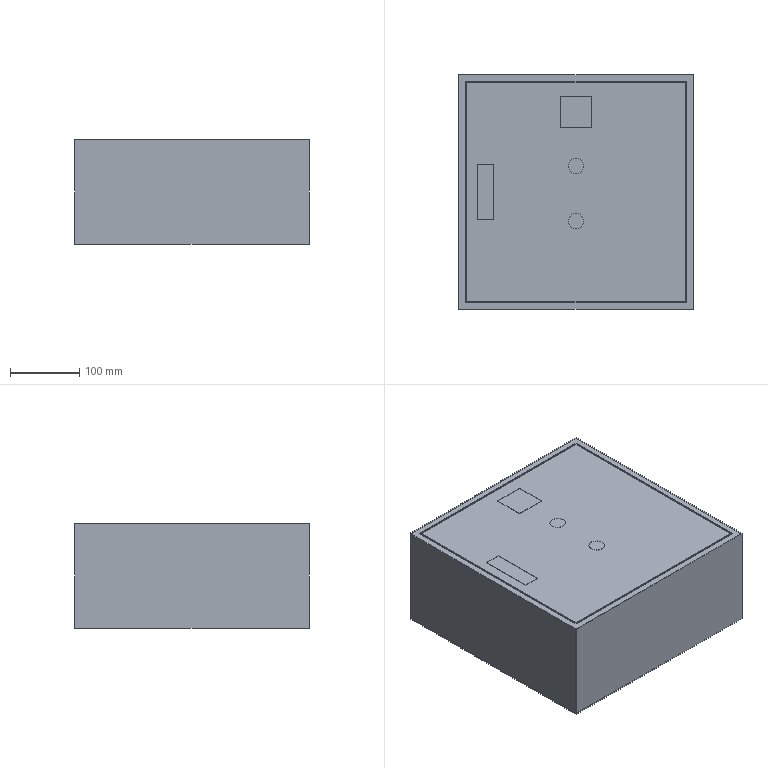Part | SolidWorks | features ICE 2, Extrusion 1, Shell 1 | 1 solid | 38 faces | box 340 x 340 x 151 mm | volume 586961 mm3 | plane 34 | cylinder 4 | commonest cylinder face diameters 22.5 x4
STEP:
#1=CARTESIAN_POINT('',(158.75,127.5,150.5));
#2=VERTEX_POINT('',#1);
#3=CARTESIAN_POINT('',(181.25,127.5,150.5));
#4=VERTEX_POINT('',#3);
#5=CARTESIAN_POINT('',(170.,127.5,150.5));
#6=DIRECTION('',(0.,0.,1.));
#7=DIRECTION('',(1.,0.,0.));
#8=AXIS2_PLACEMENT_3D('',#5,#6,#7);
#9=CIRCLE('',#8,11.25);
#10=EDGE_CURVE('',#2,#4,#9,.T.);
#11=ORIENTED_EDGE('',*,*,#10,.F.);
#12=CARTESIAN_POINT('',(158.75,127.5,151.));
#13=VERTEX_POINT('',#12);
#14=CARTESIAN_POINT('',(158.75,127.5,150.5));
#15=DIRECTION('',(0.,0.,1.));
#16=VECTOR('',#15,1000.);
#17=LINE('',#14,#16);
#18=EDGE_CURVE('',#2,#13,#17,.T.);
#19=ORIENTED_EDGE('',*,*,#18,.T.);
#20=CARTESIAN_POINT('',(181.25,127.5,151.));
#21=VERTEX_POINT('',#20);
#22=CARTESIAN_POINT('',(170.,127.5,151.));
#23=DIRECTION('',(0.,0.,1.));
#24=DIRECTION('',(1.,0.,0.));
#25=AXIS2_PLACEMENT_3D('',#22,#23,#24);
#26=CIRCLE('',#25,11.25);
#27=EDGE_CURVE('',#13,#21,#26,.T.);
#28=ORIENTED_EDGE('',*,*,#27,.T.);
#29=CARTESIAN_POINT('',(181.25,127.5,150.5));
#30=DIRECTION('',(0.,0.,1.));
#31=VECTOR('',#30,1000.);
#32=LINE('',#29,#31);
#33=EDGE_CURVE('',#4,#21,#32,.T.);
#34=ORIENTED_EDGE('',*,*,#33,.F.);
#35=EDGE_LOOP('',(#11,#19,#28,#34));
#36=FACE_OUTER_BOUND('',#35,.T.);
#37=CARTESIAN_POINT('',(170.,127.5,150.5));
#38=DIRECTION('',(0.,0.,1.));
#39=DIRECTION('',(1.,0.,0.));
#40=AXIS2_PLACEMENT_3D('',#37,#38,#39);
#41=CYLINDRICAL_SURFACE('',#40,11.25);
#42=ADVANCED_FACE('',(#36),#41,.F.);
#43=CARTESIAN_POINT('',(158.75,207.5,150.5));
#44=VERTEX_POINT('',#43);
#45=CARTESIAN_POINT('',(181.25,207.5,150.5));
#46=VERTEX_POINT('',#45);
#47=CARTESIAN_POINT('',(170.,207.5,150.5));
#48=DIRECTION('',(0.,0.,1.));
#49=DIRECTION('',(1.,0.,0.));
#50=AXIS2_PLACEMENT_3D('',#47,#48,#49);
#51=CIRCLE('',#50,11.25);
#52=EDGE_CURVE('',#44,#46,#51,.T.);
#53=ORIENTED_EDGE('',*,*,#52,.F.);
#54=CARTESIAN_POINT('',(158.75,207.5,151.));
#55=VERTEX_POINT('',#54);
#56=CARTESIAN_POINT('',(158.75,207.5,150.5));
#57=DIRECTION('',(0.,0.,1.));
#58=VECTOR('',#57,1000.);
#59=LINE('',#56,#58);
#60=EDGE_CURVE('',#44,#55,#59,.T.);
#61=ORIENTED_EDGE('',*,*,#60,.T.);
#62=CARTESIAN_POINT('',(181.25,207.5,151.));
#63=VERTEX_POINT('',#62);
#64=CARTESIAN_POINT('',(170.,207.5,151.));
#65=DIRECTION('',(0.,0.,1.));
#66=DIRECTION('',(1.,0.,0.));
#67=AXIS2_PLACEMENT_3D('',#64,#65,#66);
#68=CIRCLE('',#67,11.25);
#69=EDGE_CURVE('',#55,#63,#68,.T.);
#70=ORIENTED_EDGE('',*,*,#69,.T.);
#71=CARTESIAN_POINT('',(181.25,207.5,150.5));
#72=DIRECTION('',(0.,0.,1.));
#73=VECTOR('',#72,1000.);
#74=LINE('',#71,#73);
#75=EDGE_CURVE('',#46,#63,#74,.T.);
#76=ORIENTED_EDGE('',*,*,#75,.F.);
#77=EDGE_LOOP('',(#53,#61,#70,#76));
#78=FACE_OUTER_BOUND('',#77,.T.);
#79=CARTESIAN_POINT('',(170.,207.5,150.5));
#80=DIRECTION('',(0.,0.,1.));
#81=DIRECTION('',(1.,0.,0.));
#82=AXIS2_PLACEMENT_3D('',#79,#80,#81);
#83=CYLINDRICAL_SURFACE('',#82,11.25);
#84=ADVANCED_FACE('',(#78),#83,.F.);
#85=CARTESIAN_POINT('',(0.,340.,0.));
#86=VERTEX_POINT('',#85);
#87=CARTESIAN_POINT('',(0.,0.,0.));
#88=VERTEX_POINT('',#87);
#89=CARTESIAN_POINT('',(0.,0.,0.));
#90=DIRECTION('',(0.,-1.,0.));
#91=VECTOR('',#90,1000.);
#92=LINE('',#89,#91);
#93=EDGE_CURVE('',#86,#88,#92,.T.);
#94=ORIENTED_EDGE('',*,*,#93,.T.);
#95=CARTESIAN_POINT('',(0.,0.,151.));
#96=VERTEX_POINT('',#95);
#97=CARTESIAN_POINT('',(0.,0.,150.));
#98=DIRECTION('',(0.,0.,-1.));
#99=VECTOR('',#98,1000.);
#100=LINE('',#97,#99);
#101=EDGE_CURVE('',#96,#88,#100,.T.);
#102=ORIENTED_EDGE('',*,*,#101,.F.);
#103=CARTESIAN_POINT('',(0.,340.,151.));
#104=VERTEX_POINT('',#103);
#105=CARTESIAN_POINT('',(0.,340.,151.));
#106=DIRECTION('',(0.,-1.,0.));
#107=VECTOR('',#106,1000.);
#108=LINE('',#105,#107);
#109=EDGE_CURVE('',#104,#96,#108,.T.);
#110=ORIENTED_EDGE('',*,*,#109,.F.);
#111=CARTESIAN_POINT('',(0.,340.,150.));
#112=DIRECTION('',(0.,0.,-1.));
#113=VECTOR('',#112,1000.);
#114=LINE('',#111,#113);
#115=EDGE_CURVE('',#104,#86,#114,.T.);
#116=ORIENTED_EDGE('',*,*,#115,.T.);
#117=EDGE_LOOP('',(#94,#102,#110,#116));
#118=FACE_OUTER_BOUND('',#117,.T.);
#119=CARTESIAN_POINT('',(0.,0.,150.));
#120=DIRECTION('',(1.,0.,0.));
#121=DIRECTION('',(0.,0.,-1.));
#122=AXIS2_PLACEMENT_3D('',#119,#120,#121);
#123=PLANE('',#122);
#124=ADVANCED_FACE('',(#118),#123,.F.);
#125=CARTESIAN_POINT('',(340.,0.,0.));
#126=VERTEX_POINT('',#125);
#127=CARTESIAN_POINT('',(0.,0.,0.));
#128=DIRECTION('',(1.,0.,0.));
#129=VECTOR('',#128,1000.);
#130=LINE('',#127,#129);
#131=EDGE_CURVE('',#88,#126,#130,.T.);
#132=ORIENTED_EDGE('',*,*,#131,.T.);
#133=CARTESIAN_POINT('',(340.,0.,151.));
#134=VERTEX_POINT('',#133);
#135=CARTESIAN_POINT('',(340.,0.,150.));
#136=DIRECTION('',(0.,0.,-1.));
#137=VECTOR('',#136,1000.);
#138=LINE('',#135,#137);
#139=EDGE_CURVE('',#134,#126,#138,.T.);
#140=ORIENTED_EDGE('',*,*,#139,.F.);
#141=CARTESIAN_POINT('',(0.,0.,151.));
#142=DIRECTION('',(1.,0.,0.));
#143=VECTOR('',#142,1000.);
#144=LINE('',#141,#143);
#145=EDGE_CURVE('',#96,#134,#144,.T.);
#146=ORIENTED_EDGE('',*,*,#145,.F.);
#147=ORIENTED_EDGE('',*,*,#101,.T.);
#148=EDGE_LOOP('',(#132,#140,#146,#147));
#149=FACE_OUTER_BOUND('',#148,.T.);
#150=CARTESIAN_POINT('',(0.,0.,150.));
#151=DIRECTION('',(0.,1.,0.));
#152=DIRECTION('',(0.,0.,1.));
#153=AXIS2_PLACEMENT_3D('',#150,#151,#152);
#154=PLANE('',#153);
#155=ADVANCED_FACE('',(#149),#154,.F.);
#156=CARTESIAN_POINT('',(340.,340.,0.));
#157=VERTEX_POINT('',#156);
#158=CARTESIAN_POINT('',(340.,0.,0.));
#159=DIRECTION('',(0.,1.,0.));
#160=VECTOR('',#159,1000.);
#161=LINE('',#158,#160);
#162=EDGE_CURVE('',#126,#157,#161,.T.);
#163=ORIENTED_EDGE('',*,*,#162,.T.);
#164=CARTESIAN_POINT('',(340.,340.,151.));
#165=VERTEX_POINT('',#164);
#166=CARTESIAN_POINT('',(340.,340.,150.));
#167=DIRECTION('',(0.,0.,-1.));
#168=VECTOR('',#167,1000.);
#169=LINE('',#166,#168);
#170=EDGE_CURVE('',#165,#157,#169,.T.);
#171=ORIENTED_EDGE('',*,*,#170,.F.);
#172=CARTESIAN_POINT('',(340.,0.,151.));
#173=DIRECTION('',(0.,1.,0.));
#174=VECTOR('',#173,1000.);
#175=LINE('',#172,#174);
#176=EDGE_CURVE('',#134,#165,#175,.T.);
#177=ORIENTED_EDGE('',*,*,#176,.F.);
#178=ORIENTED_EDGE('',*,*,#139,.T.);
#179=EDGE_LOOP('',(#163,#171,#177,#178));
#180=FACE_OUTER_BOUND('',#179,.T.);
#181=CARTESIAN_POINT('',(340.,0.,150.));
#182=DIRECTION('',(-1.,0.,0.));
#183=DIRECTION('',(0.,0.,1.));
#184=AXIS2_PLACEMENT_3D('',#181,#182,#183);
#185=PLANE('',#184);
#186=ADVANCED_FACE('',(#180),#185,.F.);
#187=CARTESIAN_POINT('',(0.,340.,0.));
#188=DIRECTION('',(-1.,0.,0.));
#189=VECTOR('',#188,1000.);
#190=LINE('',#187,#189);
#191=EDGE_CURVE('',#157,#86,#190,.T.);
#192=ORIENTED_EDGE('',*,*,#191,.T.);
#193=ORIENTED_EDGE('',*,*,#115,.F.);
#194=CARTESIAN_POINT('',(340.,340.,151.));
#195=DIRECTION('',(-1.,0.,0.));
#196=VECTOR('',#195,1000.);
#197=LINE('',#194,#196);
#198=EDGE_CURVE('',#165,#104,#197,.T.);
#199=ORIENTED_EDGE('',*,*,#198,.F.);
#200=ORIENTED_EDGE('',*,*,#170,.T.);
#201=EDGE_LOOP('',(#192,#193,#199,#200));
#202=FACE_OUTER_BOUND('',#201,.T.);
#203=CARTESIAN_POINT('',(0.,340.,150.));
#204=DIRECTION('',(0.,-1.,0.));
#205=DIRECTION('',(0.,0.,-1.));
#206=AXIS2_PLACEMENT_3D('',#203,#204,#205);
#207=PLANE('',#206);
#208=ADVANCED_FACE('',(#202),#207,.F.);
#209=ORIENTED_EDGE('',*,*,#93,.F.);
#210=ORIENTED_EDGE('',*,*,#191,.F.);
#211=ORIENTED_EDGE('',*,*,#162,.F.);
#212=ORIENTED_EDGE('',*,*,#131,.F.);
#213=EDGE_LOOP('',(#209,#210,#211,#212));
#214=FACE_OUTER_BOUND('',#213,.T.);
#215=CARTESIAN_POINT('',(0.,0.,0.));
#216=DIRECTION('',(0.,0.,-1.));
#217=DIRECTION('',(-1.,0.,0.));
#218=AXIS2_PLACEMENT_3D('',#215,#216,#217);
#219=PLANE('',#218);
#220=ADVANCED_FACE('',(#214),#219,.T.);
#221=CARTESIAN_POINT('',(330.,330.,151.));
#222=VERTEX_POINT('',#221);
#223=CARTESIAN_POINT('',(10.,330.,151.));
#224=VERTEX_POINT('',#223);
#225=CARTESIAN_POINT('',(0.,330.,151.));
#226=DIRECTION('',(-1.,0.,0.));
#227=VECTOR('',#226,1000.);
#228=LINE('',#225,#227);
#229=EDGE_CURVE('',#222,#224,#228,.T.);
#230=ORIENTED_EDGE('',*,*,#229,.F.);
#231=CARTESIAN_POINT('',(330.,10.,151.));
#232=VERTEX_POINT('',#231);
#233=CARTESIAN_POINT('',(330.,0.,151.));
#234=DIRECTION('',(0.,1.,0.));
#235=VECTOR('',#234,1000.);
#236=LINE('',#233,#235);
#237=EDGE_CURVE('',#232,#222,#236,.T.);
#238=ORIENTED_EDGE('',*,*,#237,.F.);
#239=CARTESIAN_POINT('',(10.,10.,151.));
#240=VERTEX_POINT('',#239);
#241=CARTESIAN_POINT('',(0.,10.,151.));
#242=DIRECTION('',(1.,0.,0.));
#243=VECTOR('',#242,1000.);
#244=LINE('',#241,#243);
#245=EDGE_CURVE('',#240,#232,#244,.T.);
#246=ORIENTED_EDGE('',*,*,#245,.F.);
#247=CARTESIAN_POINT('',(10.,0.,151.));
#248=DIRECTION('',(0.,-1.,0.));
#249=VECTOR('',#248,1000.);
#250=LINE('',#247,#249);
#251=EDGE_CURVE('',#224,#240,#250,.T.);
#252=ORIENTED_EDGE('',*,*,#251,.F.);
#253=EDGE_LOOP('',(#230,#238,#246,#252));
#254=FACE_BOUND('',#253,.T.);
#255=ORIENTED_EDGE('',*,*,#198,.T.);
#256=ORIENTED_EDGE('',*,*,#109,.T.);
#257=ORIENTED_EDGE('',*,*,#145,.T.);
#258=ORIENTED_EDGE('',*,*,#176,.T.);
#259=EDGE_LOOP('',(#255,#256,#257,#258));
#260=FACE_OUTER_BOUND('',#259,.T.);
#261=CARTESIAN_POINT('',(0.,0.,151.));
#262=DIRECTION('',(0.,0.,1.));
#263=DIRECTION('',(1.,0.,0.));
#264=AXIS2_PLACEMENT_3D('',#261,#262,#263);
#265=PLANE('',#264);
#266=ADVANCED_FACE('',(#254,#260),#265,.T.);
#267=ORIENTED_EDGE('',*,*,#229,.T.);
#268=CARTESIAN_POINT('',(10.,330.,150.5));
#269=VERTEX_POINT('',#268);
#270=CARTESIAN_POINT('',(10.,330.,150.5));
#271=DIRECTION('',(0.,0.,1.));
#272=VECTOR('',#271,1000.);
#273=LINE('',#270,#272);
#274=EDGE_CURVE('',#269,#224,#273,.T.);
#275=ORIENTED_EDGE('',*,*,#274,.F.);
#276=CARTESIAN_POINT('',(330.,330.,150.5));
#277=VERTEX_POINT('',#276);
#278=CARTESIAN_POINT('',(0.,330.,150.5));
#279=DIRECTION('',(-1.,0.,0.));
#280=VECTOR('',#279,1000.);
#281=LINE('',#278,#280);
#282=EDGE_CURVE('',#277,#269,#281,.T.);
#283=ORIENTED_EDGE('',*,*,#282,.F.);
#284=CARTESIAN_POINT('',(330.,330.,150.5));
#285=DIRECTION('',(0.,0.,1.));
#286=VECTOR('',#285,1000.);
#287=LINE('',#284,#286);
#288=EDGE_CURVE('',#277,#222,#287,.T.);
#289=ORIENTED_EDGE('',*,*,#288,.T.);
#290=EDGE_LOOP('',(#267,#275,#283,#289));
#291=FACE_OUTER_BOUND('',#290,.T.);
#292=CARTESIAN_POINT('',(0.,330.,150.5));
#293=DIRECTION('',(0.,1.,0.));
#294=DIRECTION('',(0.,0.,1.));
#295=AXIS2_PLACEMENT_3D('',#292,#293,#294);
#296=PLANE('',#295);
#297=ADVANCED_FACE('',(#291),#296,.F.);
#298=ORIENTED_EDGE('',*,*,#237,.T.);
#299=ORIENTED_EDGE('',*,*,#288,.F.);
#300=CARTESIAN_POINT('',(330.,10.,150.5));
#301=VERTEX_POINT('',#300);
#302=CARTESIAN_POINT('',(330.,0.,150.5));
#303=DIRECTION('',(0.,1.,0.));
#304=VECTOR('',#303,1000.);
#305=LINE('',#302,#304);
#306=EDGE_CURVE('',#301,#277,#305,.T.);
#307=ORIENTED_EDGE('',*,*,#306,.F.);
#308=CARTESIAN_POINT('',(330.,10.,150.5));
#309=DIRECTION('',(0.,0.,1.));
#310=VECTOR('',#309,1000.);
#311=LINE('',#308,#310);
#312=EDGE_CURVE('',#301,#232,#311,.T.);
#313=ORIENTED_EDGE('',*,*,#312,.T.);
#314=EDGE_LOOP('',(#298,#299,#307,#313));
#315=FACE_OUTER_BOUND('',#314,.T.);
#316=CARTESIAN_POINT('',(330.,0.,150.5));
#317=DIRECTION('',(1.,0.,0.));
#318=DIRECTION('',(0.,0.,-1.));
#319=AXIS2_PLACEMENT_3D('',#316,#317,#318);
#320=PLANE('',#319);
#321=ADVANCED_FACE('',(#315),#320,.F.);
#322=ORIENTED_EDGE('',*,*,#245,.T.);
#323=ORIENTED_EDGE('',*,*,#312,.F.);
#324=CARTESIAN_POINT('',(10.,10.,150.5));
#325=VERTEX_POINT('',#324);
#326=CARTESIAN_POINT('',(0.,10.,150.5));
#327=DIRECTION('',(1.,0.,0.));
#328=VECTOR('',#327,1000.);
#329=LINE('',#326,#328);
#330=EDGE_CURVE('',#325,#301,#329,.T.);
#331=ORIENTED_EDGE('',*,*,#330,.F.);
#332=CARTESIAN_POINT('',(10.,10.,150.5));
#333=DIRECTION('',(0.,0.,1.));
#334=VECTOR('',#333,1000.);
#335=LINE('',#332,#334);
#336=EDGE_CURVE('',#325,#240,#335,.T.);
#337=ORIENTED_EDGE('',*,*,#336,.T.);
#338=EDGE_LOOP('',(#322,#323,#331,#337));
#339=FACE_OUTER_BOUND('',#338,.T.);
#340=CARTESIAN_POINT('',(0.,10.,150.5));
#341=DIRECTION('',(0.,-1.,0.));
#342=DIRECTION('',(0.,0.,-1.));
#343=AXIS2_PLACEMENT_3D('',#340,#341,#342);
#344=PLANE('',#343);
#345=ADVANCED_FACE('',(#339),#344,.F.);
#346=CARTESIAN_POINT('',(328.,12.,151.));
#347=VERTEX_POINT('',#346);
#348=CARTESIAN_POINT('',(328.,328.,151.));
#349=VERTEX_POINT('',#348);
#350=CARTESIAN_POINT('',(328.,0.,151.));
#351=DIRECTION('',(0.,1.,0.));
#352=VECTOR('',#351,1000.);
#353=LINE('',#350,#352);
#354=EDGE_CURVE('',#347,#349,#353,.T.);
#355=ORIENTED_EDGE('',*,*,#354,.F.);
#356=CARTESIAN_POINT('',(328.,12.,150.5));
#357=VERTEX_POINT('',#356);
#358=CARTESIAN_POINT('',(328.,12.,150.5));
#359=DIRECTION('',(0.,0.,1.));
#360=VECTOR('',#359,1000.);
#361=LINE('',#358,#360);
#362=EDGE_CURVE('',#357,#347,#361,.T.);
#363=ORIENTED_EDGE('',*,*,#362,.F.);
#364=CARTESIAN_POINT('',(328.,328.,150.5));
#365=VERTEX_POINT('',#364);
#366=CARTESIAN_POINT('',(328.,0.,150.5));
#367=DIRECTION('',(0.,1.,0.));
#368=VECTOR('',#367,1000.);
#369=LINE('',#366,#368);
#370=EDGE_CURVE('',#357,#365,#369,.T.);
#371=ORIENTED_EDGE('',*,*,#370,.T.);
#372=CARTESIAN_POINT('',(328.,328.,150.5));
#373=DIRECTION('',(0.,0.,1.));
#374=VECTOR('',#373,1000.);
#375=LINE('',#372,#374);
#376=EDGE_CURVE('',#365,#349,#375,.T.);
#377=ORIENTED_EDGE('',*,*,#376,.T.);
#378=EDGE_LOOP('',(#355,#363,#371,#377));
#379=FACE_OUTER_BOUND('',#378,.T.);
#380=CARTESIAN_POINT('',(328.,0.,150.5));
#381=DIRECTION('',(1.,0.,0.));
#382=DIRECTION('',(0.,0.,-1.));
#383=AXIS2_PLACEMENT_3D('',#380,#381,#382);
#384=PLANE('',#383);
#385=ADVANCED_FACE('',(#379),#384,.T.);
#386=CARTESIAN_POINT('',(12.,328.,151.));
#387=VERTEX_POINT('',#386);
#388=CARTESIAN_POINT('',(0.,328.,151.));
#389=DIRECTION('',(-1.,0.,0.));
#390=VECTOR('',#389,1000.);
#391=LINE('',#388,#390);
#392=EDGE_CURVE('',#349,#387,#391,.T.);
#393=ORIENTED_EDGE('',*,*,#392,.F.);
#394=ORIENTED_EDGE('',*,*,#376,.F.);
#395=CARTESIAN_POINT('',(12.,328.,150.5));
#396=VERTEX_POINT('',#395);
#397=CARTESIAN_POINT('',(0.,328.,150.5));
#398=DIRECTION('',(-1.,0.,0.));
#399=VECTOR('',#398,1000.);
#400=LINE('',#397,#399);
#401=EDGE_CURVE('',#365,#396,#400,.T.);
#402=ORIENTED_EDGE('',*,*,#401,.T.);
#403=CARTESIAN_POINT('',(12.,328.,150.5));
#404=DIRECTION('',(0.,0.,1.));
#405=VECTOR('',#404,1000.);
#406=LINE('',#403,#405);
#407=EDGE_CURVE('',#396,#387,#406,.T.);
#408=ORIENTED_EDGE('',*,*,#407,.T.);
#409=EDGE_LOOP('',(#393,#394,#402,#408));
#410=FACE_OUTER_BOUND('',#409,.T.);
#411=CARTESIAN_POINT('',(0.,328.,150.5));
#412=DIRECTION('',(0.,1.,0.));
#413=DIRECTION('',(0.,0.,1.));
#414=AXIS2_PLACEMENT_3D('',#411,#412,#413);
#415=PLANE('',#414);
#416=ADVANCED_FACE('',(#410),#415,.T.);
#417=CARTESIAN_POINT('',(12.,12.,151.));
#418=VERTEX_POINT('',#417);
#419=CARTESIAN_POINT('',(12.,0.,151.));
#420=DIRECTION('',(0.,-1.,0.));
#421=VECTOR('',#420,1000.);
#422=LINE('',#419,#421);
#423=EDGE_CURVE('',#387,#418,#422,.T.);
#424=ORIENTED_EDGE('',*,*,#423,.F.);
#425=ORIENTED_EDGE('',*,*,#407,.F.);
#426=CARTESIAN_POINT('',(12.,12.,150.5));
#427=VERTEX_POINT('',#426);
#428=CARTESIAN_POINT('',(12.,0.,150.5));
#429=DIRECTION('',(0.,-1.,0.));
#430=VECTOR('',#429,1000.);
#431=LINE('',#428,#430);
#432=EDGE_CURVE('',#396,#427,#431,.T.);
#433=ORIENTED_EDGE('',*,*,#432,.T.);
#434=CARTESIAN_POINT('',(12.,12.,150.5));
#435=DIRECTION('',(0.,0.,1.));
#436=VECTOR('',#435,1000.);
#437=LINE('',#434,#436);
#438=EDGE_CURVE('',#427,#418,#437,.T.);
#439=ORIENTED_EDGE('',*,*,#438,.T.);
#440=EDGE_LOOP('',(#424,#425,#433,#439));
#441=FACE_OUTER_BOUND('',#440,.T.);
#442=CARTESIAN_POINT('',(12.,0.,150.5));
#443=DIRECTION('',(-1.,0.,0.));
#444=DIRECTION('',(0.,0.,1.));
#445=AXIS2_PLACEMENT_3D('',#442,#443,#444);
#446=PLANE('',#445);
#447=ADVANCED_FACE('',(#441),#446,.T.);
#448=CARTESIAN_POINT('',(0.,12.,151.));
#449=DIRECTION('',(1.,0.,0.));
#450=VECTOR('',#449,1000.);
#451=LINE('',#448,#450);
#452=EDGE_CURVE('',#418,#347,#451,.T.);
#453=ORIENTED_EDGE('',*,*,#452,.F.);
#454=ORIENTED_EDGE('',*,*,#438,.F.);
#455=CARTESIAN_POINT('',(0.,12.,150.5));
#456=DIRECTION('',(1.,0.,0.));
#457=VECTOR('',#456,1000.);
#458=LINE('',#455,#457);
#459=EDGE_CURVE('',#427,#357,#458,.T.);
#460=ORIENTED_EDGE('',*,*,#459,.T.);
#461=ORIENTED_EDGE('',*,*,#362,.T.);
#462=EDGE_LOOP('',(#453,#454,#460,#461));
#463=FACE_OUTER_BOUND('',#462,.T.);
#464=CARTESIAN_POINT('',(0.,12.,150.5));
#465=DIRECTION('',(0.,-1.,0.));
#466=DIRECTION('',(1.,0.,0.));
#467=AXIS2_PLACEMENT_3D('',#464,#465,#466);
#468=PLANE('',#467);
#469=ADVANCED_FACE('',(#463),#468,.T.);
#470=ORIENTED_EDGE('',*,*,#251,.T.);
#471=ORIENTED_EDGE('',*,*,#336,.F.);
#472=CARTESIAN_POINT('',(10.,0.,150.5));
#473=DIRECTION('',(0.,-1.,0.));
#474=VECTOR('',#473,1000.);
#475=LINE('',#472,#474);
#476=EDGE_CURVE('',#269,#325,#475,.T.);
#477=ORIENTED_EDGE('',*,*,#476,.F.);
#478=ORIENTED_EDGE('',*,*,#274,.T.);
#479=EDGE_LOOP('',(#470,#471,#477,#478));
#480=FACE_OUTER_BOUND('',#479,.T.);
#481=CARTESIAN_POINT('',(10.,0.,150.5));
#482=DIRECTION('',(-1.,0.,0.));
#483=DIRECTION('',(0.,0.,1.));
#484=AXIS2_PLACEMENT_3D('',#481,#482,#483);
#485=PLANE('',#484);
#486=ADVANCED_FACE('',(#480),#485,.F.);
#487=ORIENTED_EDGE('',*,*,#370,.F.);
#488=ORIENTED_EDGE('',*,*,#459,.F.);
#489=ORIENTED_EDGE('',*,*,#432,.F.);
#490=ORIENTED_EDGE('',*,*,#401,.F.);
#491=EDGE_LOOP('',(#487,#488,#489,#490));
#492=FACE_BOUND('',#491,.T.);
#493=ORIENTED_EDGE('',*,*,#282,.T.);
#494=ORIENTED_EDGE('',*,*,#476,.T.);
#495=ORIENTED_EDGE('',*,*,#330,.T.);
#496=ORIENTED_EDGE('',*,*,#306,.T.);
#497=EDGE_LOOP('',(#493,#494,#495,#496));
#498=FACE_OUTER_BOUND('',#497,.T.);
#499=CARTESIAN_POINT('',(0.,0.,150.5));
#500=DIRECTION('',(0.,0.,1.));
#501=DIRECTION('',(1.,0.,0.));
#502=AXIS2_PLACEMENT_3D('',#499,#500,#501);
#503=PLANE('',#502);
#504=ADVANCED_FACE('',(#492,#498),#503,.T.);
#505=CARTESIAN_POINT('',(147.5,263.,151.));
#506=VERTEX_POINT('',#505);
#507=CARTESIAN_POINT('',(192.5,263.,151.));
#508=VERTEX_POINT('',#507);
#509=CARTESIAN_POINT('',(0.,263.,151.));
#510=DIRECTION('',(1.,0.,0.));
#511=VECTOR('',#510,1000.);
#512=LINE('',#509,#511);
#513=EDGE_CURVE('',#506,#508,#512,.T.);
#514=ORIENTED_EDGE('',*,*,#513,.F.);
#515=CARTESIAN_POINT('',(147.5,308.,151.));
#516=VERTEX_POINT('',#515);
#517=CARTESIAN_POINT('',(147.5,0.,151.));
#518=DIRECTION('',(0.,1.,0.));
#519=VECTOR('',#518,1000.);
#520=LINE('',#517,#519);
#521=EDGE_CURVE('',#506,#516,#520,.T.);
#522=ORIENTED_EDGE('',*,*,#521,.T.);
#523=CARTESIAN_POINT('',(192.5,308.,151.));
#524=VERTEX_POINT('',#523);
#525=CARTESIAN_POINT('',(0.,308.,151.));
#526=DIRECTION('',(1.,0.,0.));
#527=VECTOR('',#526,1000.);
#528=LINE('',#525,#527);
#529=EDGE_CURVE('',#516,#524,#528,.T.);
#530=ORIENTED_EDGE('',*,*,#529,.T.);
#531=CARTESIAN_POINT('',(192.5,0.,151.));
#532=DIRECTION('',(0.,1.,0.));
#533=VECTOR('',#532,1000.);
#534=LINE('',#531,#533);
#535=EDGE_CURVE('',#508,#524,#534,.T.);
#536=ORIENTED_EDGE('',*,*,#535,.F.);
#537=EDGE_LOOP('',(#514,#522,#530,#536));
#538=FACE_BOUND('',#537,.T.);
#539=CARTESIAN_POINT('',(170.,127.5,151.));
#540=DIRECTION('',(0.,0.,1.));
#541=DIRECTION('',(1.,0.,0.));
#542=AXIS2_PLACEMENT_3D('',#539,#540,#541);
#543=CIRCLE('',#542,11.25);
#544=EDGE_CURVE('',#21,#13,#543,.T.);
#545=ORIENTED_EDGE('',*,*,#544,.F.);
#546=ORIENTED_EDGE('',*,*,#27,.F.);
#547=EDGE_LOOP('',(#545,#546));
#548=FACE_BOUND('',#547,.T.);
#549=CARTESIAN_POINT('',(170.,207.5,151.));
#550=DIRECTION('',(0.,0.,1.));
#551=DIRECTION('',(1.,0.,0.));
#552=AXIS2_PLACEMENT_3D('',#549,#550,#551);
#553=CIRCLE('',#552,11.25);
#554=EDGE_CURVE('',#63,#55,#553,.T.);
#555=ORIENTED_EDGE('',*,*,#554,.F.);
#556=ORIENTED_EDGE('',*,*,#69,.F.);
#557=EDGE_LOOP('',(#555,#556));
#558=FACE_BOUND('',#557,.T.);
#559=CARTESIAN_POINT('',(27.,130.,151.));
#560=VERTEX_POINT('',#559);
#561=CARTESIAN_POINT('',(51.,130.,151.));
#562=VERTEX_POINT('',#561);
#563=CARTESIAN_POINT('',(0.,130.,151.));
#564=DIRECTION('',(1.,0.,0.));
#565=VECTOR('',#564,1000.);
#566=LINE('',#563,#565);
#567=EDGE_CURVE('',#560,#562,#566,.T.);
#568=ORIENTED_EDGE('',*,*,#567,.F.);
#569=CARTESIAN_POINT('',(27.,210.,151.));
#570=VERTEX_POINT('',#569);
#571=CARTESIAN_POINT('',(27.,0.,151.));
#572=DIRECTION('',(0.,1.,0.));
#573=VECTOR('',#572,1000.);
#574=LINE('',#571,#573);
#575=EDGE_CURVE('',#560,#570,#574,.T.);
#576=ORIENTED_EDGE('',*,*,#575,.T.);
#577=CARTESIAN_POINT('',(51.,210.,151.));
#578=VERTEX_POINT('',#577);
#579=CARTESIAN_POINT('',(0.,210.,151.));
#580=DIRECTION('',(1.,0.,0.));
#581=VECTOR('',#580,1000.);
#582=LINE('',#579,#581);
#583=EDGE_CURVE('',#570,#578,#582,.T.);
#584=ORIENTED_EDGE('',*,*,#583,.T.);
#585=CARTESIAN_POINT('',(51.,0.,151.));
#586=DIRECTION('',(0.,1.,0.));
#587=VECTOR('',#586,1000.);
#588=LINE('',#585,#587);
#589=EDGE_CURVE('',#562,#578,#588,.T.);
#590=ORIENTED_EDGE('',*,*,#589,.F.);
#591=EDGE_LOOP('',(#568,#576,#584,#590));
#592=FACE_BOUND('',#591,.T.);
#593=ORIENTED_EDGE('',*,*,#452,.T.);
#594=ORIENTED_EDGE('',*,*,#354,.T.);
#595=ORIENTED_EDGE('',*,*,#392,.T.);
#596=ORIENTED_EDGE('',*,*,#423,.T.);
#597=EDGE_LOOP('',(#593,#594,#595,#596));
#598=FACE_OUTER_BOUND('',#597,.T.);
#599=CARTESIAN_POINT('',(0.,0.,151.));
#600=DIRECTION('',(0.,0.,1.));
#601=DIRECTION('',(1.,0.,0.));
#602=AXIS2_PLACEMENT_3D('',#599,#600,#601);
#603=PLANE('',#602);
#604=ADVANCED_FACE('',(#538,#548,#558,#592,#598),#603,.T.);
#605=ORIENTED_EDGE('',*,*,#567,.T.);
#606=CARTESIAN_POINT('',(51.,130.,150.5));
#607=VERTEX_POINT('',#606);
#608=CARTESIAN_POINT('',(51.,130.,150.5));
#609=DIRECTION('',(0.,0.,1.));
#610=VECTOR('',#609,1000.);
#611=LINE('',#608,#610);
#612=EDGE_CURVE('',#607,#562,#611,.T.);
#613=ORIENTED_EDGE('',*,*,#612,.F.);
#614=CARTESIAN_POINT('',(27.,130.,150.5));
#615=VERTEX_POINT('',#614);
#616=CARTESIAN_POINT('',(0.,130.,150.5));
#617=DIRECTION('',(1.,0.,0.));
#618=VECTOR('',#617,1000.);
#619=LINE('',#616,#618);
#620=EDGE_CURVE('',#615,#607,#619,.T.);
#621=ORIENTED_EDGE('',*,*,#620,.F.);
#622=CARTESIAN_POINT('',(27.,130.,150.5));
#623=DIRECTION('',(0.,0.,1.));
#624=VECTOR('',#623,1000.);
#625=LINE('',#622,#624);
#626=EDGE_CURVE('',#615,#560,#625,.T.);
#627=ORIENTED_EDGE('',*,*,#626,.T.);
#628=EDGE_LOOP('',(#605,#613,#621,#627));
#629=FACE_OUTER_BOUND('',#628,.T.);
#630=CARTESIAN_POINT('',(0.,130.,150.5));
#631=DIRECTION('',(0.,-1.,0.));
#632=DIRECTION('',(0.,0.,-1.));
#633=AXIS2_PLACEMENT_3D('',#630,#631,#632);
#634=PLANE('',#633);
#635=ADVANCED_FACE('',(#629),#634,.F.);
#636=ORIENTED_EDGE('',*,*,#575,.F.);
#637=ORIENTED_EDGE('',*,*,#626,.F.);
#638=CARTESIAN_POINT('',(27.,210.,150.5));
#639=VERTEX_POINT('',#638);
#640=CARTESIAN_POINT('',(27.,0.,150.5));
#641=DIRECTION('',(0.,1.,0.));
#642=VECTOR('',#641,1000.);
#643=LINE('',#640,#642);
#644=EDGE_CURVE('',#615,#639,#643,.T.);
#645=ORIENTED_EDGE('',*,*,#644,.T.);
#646=CARTESIAN_POINT('',(27.,210.,150.5));
#647=DIRECTION('',(0.,0.,1.));
#648=VECTOR('',#647,1000.);
#649=LINE('',#646,#648);
#650=EDGE_CURVE('',#639,#570,#649,.T.);
#651=ORIENTED_EDGE('',*,*,#650,.T.);
#652=EDGE_LOOP('',(#636,#637,#645,#651));
#653=FACE_OUTER_BOUND('',#652,.T.);
#654=CARTESIAN_POINT('',(27.,0.,150.5));
#655=DIRECTION('',(1.,0.,0.));
#656=DIRECTION('',(0.,1.,0.));
#657=AXIS2_PLACEMENT_3D('',#654,#655,#656);
#658=PLANE('',#657);
#659=ADVANCED_FACE('',(#653),#658,.T.);
#660=ORIENTED_EDGE('',*,*,#583,.F.);
#661=ORIENTED_EDGE('',*,*,#650,.F.);
#662=CARTESIAN_POINT('',(51.,210.,150.5));
#663=VERTEX_POINT('',#662);
#664=CARTESIAN_POINT('',(0.,210.,150.5));
#665=DIRECTION('',(1.,0.,0.));
#666=VECTOR('',#665,1000.);
#667=LINE('',#664,#666);
#668=EDGE_CURVE('',#639,#663,#667,.T.);
#669=ORIENTED_EDGE('',*,*,#668,.T.);
#670=CARTESIAN_POINT('',(51.,210.,150.5));
#671=DIRECTION('',(0.,0.,1.));
#672=VECTOR('',#671,1000.);
#673=LINE('',#670,#672);
#674=EDGE_CURVE('',#663,#578,#673,.T.);
#675=ORIENTED_EDGE('',*,*,#674,.T.);
#676=EDGE_LOOP('',(#660,#661,#669,#675));
#677=FACE_OUTER_BOUND('',#676,.T.);
#678=CARTESIAN_POINT('',(0.,210.,150.5));
#679=DIRECTION('',(0.,-1.,0.));
#680=DIRECTION('',(0.,0.,-1.));
#681=AXIS2_PLACEMENT_3D('',#678,#679,#680);
#682=PLANE('',#681);
#683=ADVANCED_FACE('',(#677),#682,.T.);
#684=ORIENTED_EDGE('',*,*,#589,.T.);
#685=ORIENTED_EDGE('',*,*,#674,.F.);
#686=CARTESIAN_POINT('',(51.,0.,150.5));
#687=DIRECTION('',(0.,1.,0.));
#688=VECTOR('',#687,1000.);
#689=LINE('',#686,#688);
#690=EDGE_CURVE('',#607,#663,#689,.T.);
#691=ORIENTED_EDGE('',*,*,#690,.F.);
#692=ORIENTED_EDGE('',*,*,#612,.T.);
#693=EDGE_LOOP('',(#684,#685,#691,#692));
#694=FACE_OUTER_BOUND('',#693,.T.);
#695=CARTESIAN_POINT('',(51.,0.,150.5));
#696=DIRECTION('',(1.,0.,0.));
#697=DIRECTION('',(0.,1.,0.));
#698=AXIS2_PLACEMENT_3D('',#695,#696,#697);
#699=PLANE('',#698);
#700=ADVANCED_FACE('',(#694),#699,.F.);
#701=ORIENTED_EDGE('',*,*,#620,.T.);
#702=ORIENTED_EDGE('',*,*,#690,.T.);
#703=ORIENTED_EDGE('',*,*,#668,.F.);
#704=ORIENTED_EDGE('',*,*,#644,.F.);
#705=EDGE_LOOP('',(#701,#702,#703,#704));
#706=FACE_OUTER_BOUND('',#705,.T.);
#707=CARTESIAN_POINT('',(0.,0.,150.5));
#708=DIRECTION('',(0.,0.,1.));
#709=DIRECTION('',(1.,0.,0.));
#710=AXIS2_PLACEMENT_3D('',#707,#708,#709);
#711=PLANE('',#710);
#712=ADVANCED_FACE('',(#706),#711,.T.);
#713=ORIENTED_EDGE('',*,*,#60,.F.);
#714=CARTESIAN_POINT('',(170.,207.5,150.5));
#715=DIRECTION('',(0.,0.,1.));
#716=DIRECTION('',(1.,0.,0.));
#717=AXIS2_PLACEMENT_3D('',#714,#715,#716);
#718=CIRCLE('',#717,11.25);
#719=EDGE_CURVE('',#46,#44,#718,.T.);
#720=ORIENTED_EDGE('',*,*,#719,.F.);
#721=ORIENTED_EDGE('',*,*,#75,.T.);
#722=ORIENTED_EDGE('',*,*,#554,.T.);
#723=EDGE_LOOP('',(#713,#720,#721,#722));
#724=FACE_OUTER_BOUND('',#723,.T.);
#725=CARTESIAN_POINT('',(170.,207.5,150.5));
#726=DIRECTION('',(0.,0.,1.));
#727=DIRECTION('',(1.,0.,0.));
#728=AXIS2_PLACEMENT_3D('',#725,#726,#727);
#729=CYLINDRICAL_SURFACE('',#728,11.25);
#730=ADVANCED_FACE('',(#724),#729,.F.);
#731=ORIENTED_EDGE('',*,*,#719,.T.);
#732=ORIENTED_EDGE('',*,*,#52,.T.);
#733=EDGE_LOOP('',(#731,#732));
#734=FACE_OUTER_BOUND('',#733,.T.);
#735=CARTESIAN_POINT('',(0.,0.,150.5));
#736=DIRECTION('',(0.,0.,1.));
#737=DIRECTION('',(1.,0.,0.));
#738=AXIS2_PLACEMENT_3D('',#735,#736,#737);
#739=PLANE('',#738);
#740=ADVANCED_FACE('',(#734),#739,.T.);
#741=ORIENTED_EDGE('',*,*,#18,.F.);
#742=CARTESIAN_POINT('',(170.,127.5,150.5));
#743=DIRECTION('',(0.,0.,1.));
#744=DIRECTION('',(1.,0.,0.));
#745=AXIS2_PLACEMENT_3D('',#742,#743,#744);
#746=CIRCLE('',#745,11.25);
#747=EDGE_CURVE('',#4,#2,#746,.T.);
#748=ORIENTED_EDGE('',*,*,#747,.F.);
#749=ORIENTED_EDGE('',*,*,#33,.T.);
#750=ORIENTED_EDGE('',*,*,#544,.T.);
#751=EDGE_LOOP('',(#741,#748,#749,#750));
#752=FACE_OUTER_BOUND('',#751,.T.);
#753=CARTESIAN_POINT('',(170.,127.5,150.5));
#754=DIRECTION('',(0.,0.,1.));
#755=DIRECTION('',(1.,0.,0.));
#756=AXIS2_PLACEMENT_3D('',#753,#754,#755);
#757=CYLINDRICAL_SURFACE('',#756,11.25);
#758=ADVANCED_FACE('',(#752),#757,.F.);
#759=ORIENTED_EDGE('',*,*,#747,.T.);
#760=ORIENTED_EDGE('',*,*,#10,.T.);
#761=EDGE_LOOP('',(#759,#760));
#762=FACE_OUTER_BOUND('',#761,.T.);
#763=CARTESIAN_POINT('',(0.,0.,150.5));
#764=DIRECTION('',(0.,0.,1.));
#765=DIRECTION('',(1.,0.,0.));
#766=AXIS2_PLACEMENT_3D('',#763,#764,#765);
#767=PLANE('',#766);
#768=ADVANCED_FACE('',(#762),#767,.T.);
#769=ORIENTED_EDGE('',*,*,#513,.T.);
#770=CARTESIAN_POINT('',(192.5,263.,150.5));
#771=VERTEX_POINT('',#770);
#772=CARTESIAN_POINT('',(192.5,263.,150.5));
#773=DIRECTION('',(0.,0.,1.));
#774=VECTOR('',#773,1000.);
#775=LINE('',#772,#774);
#776=EDGE_CURVE('',#771,#508,#775,.T.);
#777=ORIENTED_EDGE('',*,*,#776,.F.);
#778=CARTESIAN_POINT('',(147.5,263.,150.5));
#779=VERTEX_POINT('',#778);
#780=CARTESIAN_POINT('',(0.,263.,150.5));
#781=DIRECTION('',(1.,0.,0.));
#782=VECTOR('',#781,1000.);
#783=LINE('',#780,#782);
#784=EDGE_CURVE('',#779,#771,#783,.T.);
#785=ORIENTED_EDGE('',*,*,#784,.F.);
#786=CARTESIAN_POINT('',(147.5,263.,150.5));
#787=DIRECTION('',(0.,0.,1.));
#788=VECTOR('',#787,1000.);
#789=LINE('',#786,#788);
#790=EDGE_CURVE('',#779,#506,#789,.T.);
#791=ORIENTED_EDGE('',*,*,#790,.T.);
#792=EDGE_LOOP('',(#769,#777,#785,#791));
#793=FACE_OUTER_BOUND('',#792,.T.);
#794=CARTESIAN_POINT('',(0.,263.,150.5));
#795=DIRECTION('',(0.,-1.,0.));
#796=DIRECTION('',(0.,0.,-1.));
#797=AXIS2_PLACEMENT_3D('',#794,#795,#796);
#798=PLANE('',#797);
#799=ADVANCED_FACE('',(#793),#798,.F.);
#800=ORIENTED_EDGE('',*,*,#521,.F.);
#801=ORIENTED_EDGE('',*,*,#790,.F.);
#802=CARTESIAN_POINT('',(147.5,308.,150.5));
#803=VERTEX_POINT('',#802);
#804=CARTESIAN_POINT('',(147.5,0.,150.5));
#805=DIRECTION('',(0.,1.,0.));
#806=VECTOR('',#805,1000.);
#807=LINE('',#804,#806);
#808=EDGE_CURVE('',#779,#803,#807,.T.);
#809=ORIENTED_EDGE('',*,*,#808,.T.);
#810=CARTESIAN_POINT('',(147.5,308.,150.5));
#811=DIRECTION('',(0.,0.,1.));
#812=VECTOR('',#811,1000.);
#813=LINE('',#810,#812);
#814=EDGE_CURVE('',#803,#516,#813,.T.);
#815=ORIENTED_EDGE('',*,*,#814,.T.);
#816=EDGE_LOOP('',(#800,#801,#809,#815));
#817=FACE_OUTER_BOUND('',#816,.T.);
#818=CARTESIAN_POINT('',(147.5,0.,150.5));
#819=DIRECTION('',(1.,0.,0.));
#820=DIRECTION('',(0.,0.,-1.));
#821=AXIS2_PLACEMENT_3D('',#818,#819,#820);
#822=PLANE('',#821);
#823=ADVANCED_FACE('',(#817),#822,.T.);
#824=ORIENTED_EDGE('',*,*,#529,.F.);
#825=ORIENTED_EDGE('',*,*,#814,.F.);
#826=CARTESIAN_POINT('',(192.5,308.,150.5));
#827=VERTEX_POINT('',#826);
#828=CARTESIAN_POINT('',(0.,308.,150.5));
#829=DIRECTION('',(1.,0.,0.));
#830=VECTOR('',#829,1000.);
#831=LINE('',#828,#830);
#832=EDGE_CURVE('',#803,#827,#831,.T.);
#833=ORIENTED_EDGE('',*,*,#832,.T.);
#834=CARTESIAN_POINT('',(192.5,308.,150.5));
#835=DIRECTION('',(0.,0.,1.));
#836=VECTOR('',#835,1000.);
#837=LINE('',#834,#836);
#838=EDGE_CURVE('',#827,#524,#837,.T.);
#839=ORIENTED_EDGE('',*,*,#838,.T.);
#840=EDGE_LOOP('',(#824,#825,#833,#839));
#841=FACE_OUTER_BOUND('',#840,.T.);
#842=CARTESIAN_POINT('',(0.,308.,150.5));
#843=DIRECTION('',(0.,-1.,0.));
#844=DIRECTION('',(0.,0.,-1.));
#845=AXIS2_PLACEMENT_3D('',#842,#843,#844);
#846=PLANE('',#845);
#847=ADVANCED_FACE('',(#841),#846,.T.);
#848=ORIENTED_EDGE('',*,*,#535,.T.);
#849=ORIENTED_EDGE('',*,*,#838,.F.);
#850=CARTESIAN_POINT('',(192.5,0.,150.5));
#851=DIRECTION('',(0.,1.,0.));
#852=VECTOR('',#851,1000.);
#853=LINE('',#850,#852);
#854=EDGE_CURVE('',#771,#827,#853,.T.);
#855=ORIENTED_EDGE('',*,*,#854,.F.);
#856=ORIENTED_EDGE('',*,*,#776,.T.);
#857=EDGE_LOOP('',(#848,#849,#855,#856));
#858=FACE_OUTER_BOUND('',#857,.T.);
#859=CARTESIAN_POINT('',(192.5,0.,150.5));
#860=DIRECTION('',(1.,0.,0.));
#861=DIRECTION('',(0.,1.,0.));
#862=AXIS2_PLACEMENT_3D('',#859,#860,#861);
#863=PLANE('',#862);
#864=ADVANCED_FACE('',(#858),#863,.F.);
#865=ORIENTED_EDGE('',*,*,#784,.T.);
#866=ORIENTED_EDGE('',*,*,#854,.T.);
#867=ORIENTED_EDGE('',*,*,#832,.F.);
#868=ORIENTED_EDGE('',*,*,#808,.F.);
#869=EDGE_LOOP('',(#865,#866,#867,#868));
#870=FACE_OUTER_BOUND('',#869,.T.);
#871=CARTESIAN_POINT('',(0.,0.,150.5));
#872=DIRECTION('',(0.,0.,1.));
#873=DIRECTION('',(1.,0.,0.));
#874=AXIS2_PLACEMENT_3D('',#871,#872,#873);
#875=PLANE('',#874);
#876=ADVANCED_FACE('',(#870),#875,.T.);
#877=CLOSED_SHELL('',(#42,#84,#124,#155,#186,#208,#220,#266,#297,#321,#345,#385,#416,#447,#469,#486,#504,#604,#635,#659,#683,#700,#712,#730,#740,#758,#768,#799,#823,#847,#864,#876));
#878=CARTESIAN_POINT('',(1.5,338.5,1.5));
#879=VERTEX_POINT('',#878);
#880=CARTESIAN_POINT('',(1.5,1.5,1.5));
#881=VERTEX_POINT('',#880);
#882=CARTESIAN_POINT('',(1.5,0.,1.5));
#883=DIRECTION('',(0.,-1.,0.));
#884=VECTOR('',#883,1000.);
#885=LINE('',#882,#884);
#886=EDGE_CURVE('',#879,#881,#885,.T.);
#887=ORIENTED_EDGE('',*,*,#886,.T.);
#888=CARTESIAN_POINT('',(338.5,1.5,1.5));
#889=VERTEX_POINT('',#888);
#890=CARTESIAN_POINT('',(0.,1.5,1.5));
#891=DIRECTION('',(1.,0.,0.));
#892=VECTOR('',#891,1000.);
#893=LINE('',#890,#892);
#894=EDGE_CURVE('',#881,#889,#893,.T.);
#895=ORIENTED_EDGE('',*,*,#894,.T.);
#896=CARTESIAN_POINT('',(338.5,338.5,1.5));
#897=VERTEX_POINT('',#896);
#898=CARTESIAN_POINT('',(338.5,0.,1.5));
#899=DIRECTION('',(0.,1.,0.));
#900=VECTOR('',#899,1000.);
#901=LINE('',#898,#900);
#902=EDGE_CURVE('',#889,#897,#901,.T.);
#903=ORIENTED_EDGE('',*,*,#902,.T.);
#904=CARTESIAN_POINT('',(0.,338.5,1.5));
#905=DIRECTION('',(-1.,0.,0.));
#906=VECTOR('',#905,1000.);
#907=LINE('',#904,#906);
#908=EDGE_CURVE('',#897,#879,#907,.T.);
#909=ORIENTED_EDGE('',*,*,#908,.T.);
#910=EDGE_LOOP('',(#887,#895,#903,#909));
#911=FACE_OUTER_BOUND('',#910,.T.);
#912=CARTESIAN_POINT('',(0.,0.,1.5));
#913=DIRECTION('',(0.,0.,-1.));
#914=DIRECTION('',(-1.,0.,0.));
#915=AXIS2_PLACEMENT_3D('',#912,#913,#914);
#916=PLANE('',#915);
#917=ADVANCED_FACE('',(#911),#916,.F.);
#918=ORIENTED_EDGE('',*,*,#894,.F.);
#919=CARTESIAN_POINT('',(1.5,1.5,150.));
#920=VERTEX_POINT('',#919);
#921=CARTESIAN_POINT('',(1.5,1.5,150.));
#922=DIRECTION('',(0.,0.,-1.));
#923=VECTOR('',#922,1000.);
#924=LINE('',#921,#923);
#925=EDGE_CURVE('',#920,#881,#924,.T.);
#926=ORIENTED_EDGE('',*,*,#925,.F.);
#927=CARTESIAN_POINT('',(338.5,1.5,150.));
#928=VERTEX_POINT('',#927);
#929=CARTESIAN_POINT('',(0.,1.5,150.));
#930=DIRECTION('',(1.,0.,0.));
#931=VECTOR('',#930,1000.);
#932=LINE('',#929,#931);
#933=EDGE_CURVE('',#920,#928,#932,.T.);
#934=ORIENTED_EDGE('',*,*,#933,.T.);
#935=CARTESIAN_POINT('',(338.5,1.5,150.));
#936=DIRECTION('',(0.,0.,-1.));
#937=VECTOR('',#936,1000.);
#938=LINE('',#935,#937);
#939=EDGE_CURVE('',#928,#889,#938,.T.);
#940=ORIENTED_EDGE('',*,*,#939,.T.);
#941=EDGE_LOOP('',(#918,#926,#934,#940));
#942=FACE_OUTER_BOUND('',#941,.T.);
#943=CARTESIAN_POINT('',(0.,1.5,150.));
#944=DIRECTION('',(0.,1.,0.));
#945=DIRECTION('',(0.,0.,1.));
#946=AXIS2_PLACEMENT_3D('',#943,#944,#945);
#947=PLANE('',#946);
#948=ADVANCED_FACE('',(#942),#947,.T.);
#949=ORIENTED_EDGE('',*,*,#902,.F.);
#950=ORIENTED_EDGE('',*,*,#939,.F.);
#951=CARTESIAN_POINT('',(338.5,338.5,150.));
#952=VERTEX_POINT('',#951);
#953=CARTESIAN_POINT('',(338.5,0.,150.));
#954=DIRECTION('',(0.,1.,0.));
#955=VECTOR('',#954,1000.);
#956=LINE('',#953,#955);
#957=EDGE_CURVE('',#928,#952,#956,.T.);
#958=ORIENTED_EDGE('',*,*,#957,.T.);
#959=CARTESIAN_POINT('',(338.5,338.5,150.));
#960=DIRECTION('',(0.,0.,-1.));
#961=VECTOR('',#960,1000.);
#962=LINE('',#959,#961);
#963=EDGE_CURVE('',#952,#897,#962,.T.);
#964=ORIENTED_EDGE('',*,*,#963,.T.);
#965=EDGE_LOOP('',(#949,#950,#958,#964));
#966=FACE_OUTER_BOUND('',#965,.T.);
#967=CARTESIAN_POINT('',(338.5,0.,150.));
#968=DIRECTION('',(-1.,0.,0.));
#969=DIRECTION('',(0.,0.,1.));
#970=AXIS2_PLACEMENT_3D('',#967,#968,#969);
#971=PLANE('',#970);
#972=ADVANCED_FACE('',(#966),#971,.T.);
#973=ORIENTED_EDGE('',*,*,#908,.F.);
#974=ORIENTED_EDGE('',*,*,#963,.F.);
#975=CARTESIAN_POINT('',(1.5,338.5,150.));
#976=VERTEX_POINT('',#975);
#977=CARTESIAN_POINT('',(0.,338.5,150.));
#978=DIRECTION('',(-1.,0.,0.));
#979=VECTOR('',#978,1000.);
#980=LINE('',#977,#979);
#981=EDGE_CURVE('',#952,#976,#980,.T.);
#982=ORIENTED_EDGE('',*,*,#981,.T.);
#983=CARTESIAN_POINT('',(1.5,338.5,150.));
#984=DIRECTION('',(0.,0.,-1.));
#985=VECTOR('',#984,1000.);
#986=LINE('',#983,#985);
#987=EDGE_CURVE('',#976,#879,#986,.T.);
#988=ORIENTED_EDGE('',*,*,#987,.T.);
#989=EDGE_LOOP('',(#973,#974,#982,#988));
#990=FACE_OUTER_BOUND('',#989,.T.);
#991=CARTESIAN_POINT('',(0.,338.5,150.));
#992=DIRECTION('',(0.,-1.,0.));
#993=DIRECTION('',(0.,0.,-1.));
#994=AXIS2_PLACEMENT_3D('',#991,#992,#993);
#995=PLANE('',#994);
#996=ADVANCED_FACE('',(#990),#995,.T.);
#997=ORIENTED_EDGE('',*,*,#886,.F.);
#998=ORIENTED_EDGE('',*,*,#987,.F.);
#999=CARTESIAN_POINT('',(1.5,0.,150.));
#1000=DIRECTION('',(0.,-1.,0.));
#1001=VECTOR('',#1000,1000.);
#1002=LINE('',#999,#1001);
#1003=EDGE_CURVE('',#976,#920,#1002,.T.);
#1004=ORIENTED_EDGE('',*,*,#1003,.T.);
#1005=ORIENTED_EDGE('',*,*,#925,.T.);
#1006=EDGE_LOOP('',(#997,#998,#1004,#1005));
#1007=FACE_OUTER_BOUND('',#1006,.T.);
#1008=CARTESIAN_POINT('',(1.5,0.,150.));
#1009=DIRECTION('',(1.,0.,0.));
#1010=DIRECTION('',(0.,0.,-1.));
#1011=AXIS2_PLACEMENT_3D('',#1008,#1009,#1010);
#1012=PLANE('',#1011);
#1013=ADVANCED_FACE('',(#1007),#1012,.T.);
#1014=ORIENTED_EDGE('',*,*,#1003,.F.);
#1015=ORIENTED_EDGE('',*,*,#981,.F.);
#1016=ORIENTED_EDGE('',*,*,#957,.F.);
#1017=ORIENTED_EDGE('',*,*,#933,.F.);
#1018=EDGE_LOOP('',(#1014,#1015,#1016,#1017));
#1019=FACE_OUTER_BOUND('',#1018,.T.);
#1020=CARTESIAN_POINT('',(0.,0.,150.));
#1021=DIRECTION('',(0.,0.,1.));
#1022=DIRECTION('',(1.,0.,0.));
#1023=AXIS2_PLACEMENT_3D('',#1020,#1021,#1022);
#1024=PLANE('',#1023);
#1025=ADVANCED_FACE('',(#1019),#1024,.F.);
#1026=CLOSED_SHELL('',(#917,#948,#972,#996,#1013,#1025));
#1027=ORIENTED_CLOSED_SHELL('',*,#1026,.F.);
#1028=BREP_WITH_VOIDS('',#877,(#1027));
#1029=CARTESIAN_POINT('',(0.,0.,0.));
#1030=DIRECTION('',(0.,0.,1.));
#1031=DIRECTION('',(1.,0.,0.));
#1032=AXIS2_PLACEMENT_3D('',#1029,#1030,#1031);
#1033=(LENGTH_UNIT()NAMED_UNIT(*)SI_UNIT(.MILLI.,.METRE.));
#1034=UNCERTAINTY_MEASURE_WITH_UNIT(LENGTH_MEASURE(0.00001),#1033,'','');
#1035=(NAMED_UNIT(*)PLANE_ANGLE_UNIT()SI_UNIT($,.RADIAN.));
#1036=(NAMED_UNIT(*)SI_UNIT($,.STERADIAN.)SOLID_ANGLE_UNIT());
#1037=(GEOMETRIC_REPRESENTATION_CONTEXT(3)GLOBAL_UNCERTAINTY_ASSIGNED_CONTEXT((#1034))GLOBAL_UNIT_ASSIGNED_CONTEXT((#1033,#1035,#1036))REPRESENTATION_CONTEXT('',''));
#1038=ADVANCED_BREP_SHAPE_REPRESENTATION('',(#1028,#1032),#1037);